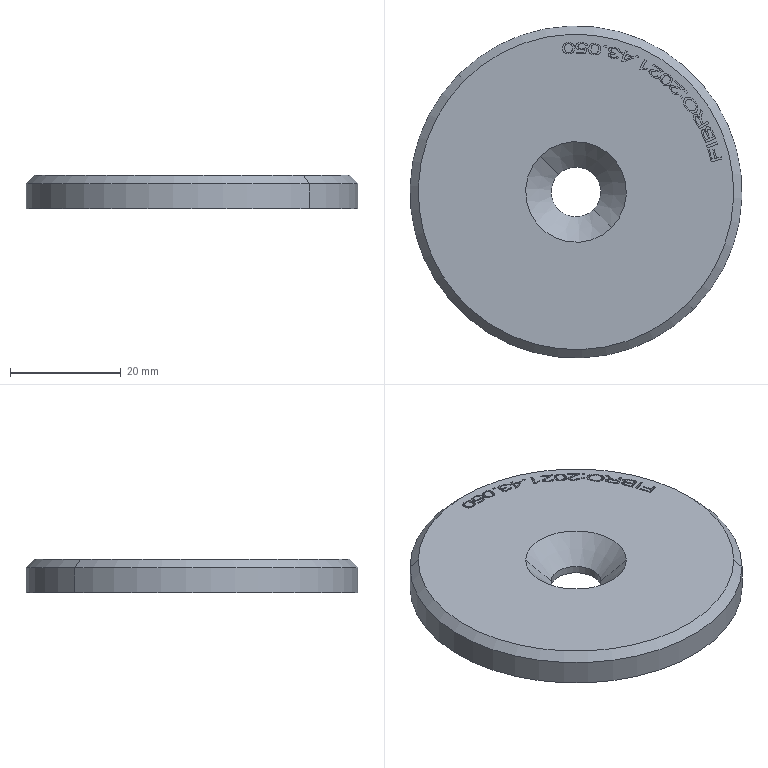Part | NX | features 1 2 | 1 solid | 206 faces | box 60 x 60 x 6 mm | volume 15960 mm3 | plane 107 | spline 91 | cylinder 4 | cone 4 | commonest cylinder face diameters 9 x2 60 x2